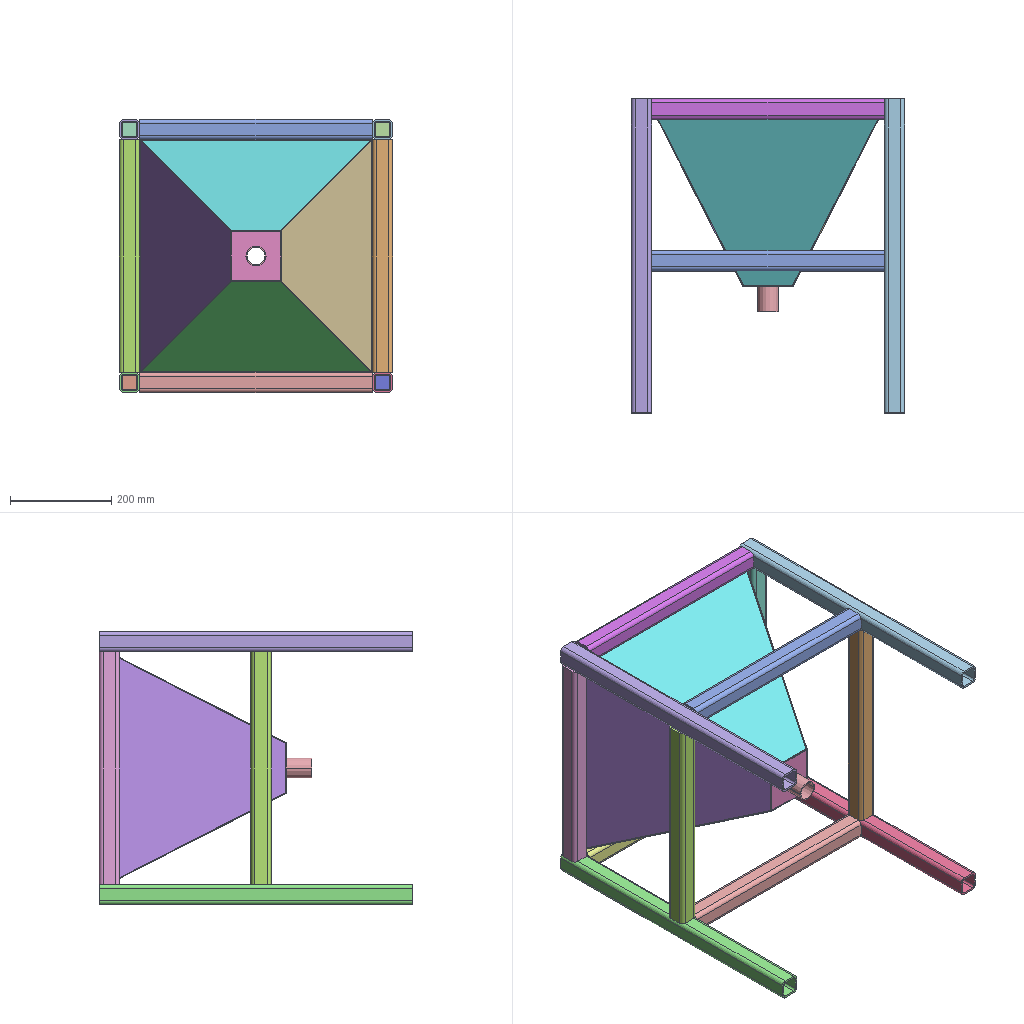Assembly | SolidWorks | 7 different items | 7 placed | box 540 x 620 x 540 mm
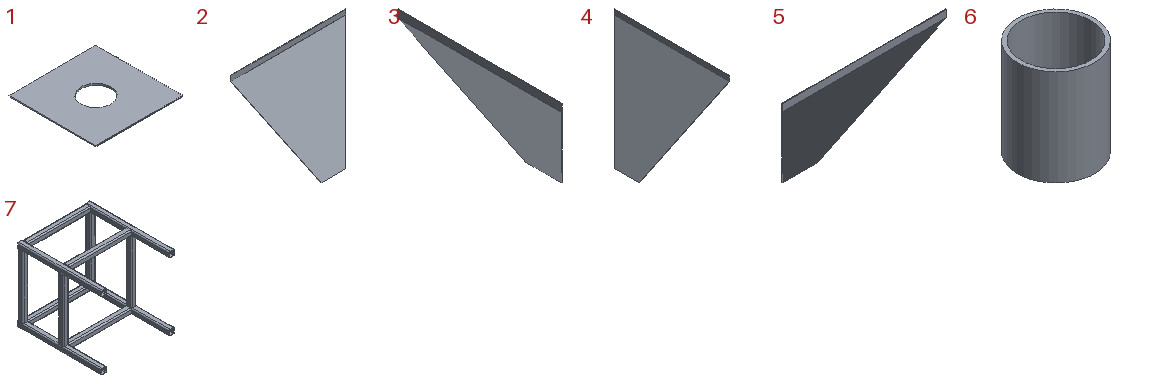Parts list (item | quantity | size | volume | features):
1 | x1 | 102.046 x 102.046 x 2 mm | 18488 mm3 | features ICE 3, DeleteBody 2, Split 2, Blend 1, Shell 1
2 | x1 | 454 x 180.224 x 368.911 mm | 234028 mm3 | features ICE 3, Blend 1, FlatPattern 1, SheetMetal 1, Shell 1, SolidToSheetMetal 1
3 | x1 | 180.781 x 458 x 370 mm | 237222 mm3 | features ICE 3, Blend 1, FlatPattern 1, SheetMetal 1, Shell 1, SolidToSheetMetal 1
4 | x1 | 180.781 x 458 x 370 mm | 237222 mm3 | features ICE 3, Blend 1, FlatPattern 1, SheetMetal 1, Shell 1, SolidToSheetMetal 1
5 | x1 | 454 x 180.224 x 368.911 mm | 234028 mm3 | features ICE 3, Blend 1, FlatPattern 1, SheetMetal 1, Shell 1, SolidToSheetMetal 1
6 | x1 | 40 x 40 x 50 mm | 11938 mm3 | features ICE 3, DeleteBody 2, Split 2, Blend 1, Shell 1
7 | x1 | 540 x 620 x 540 mm | 3300618 mm3 | features WeldCornerFeat 2, 3DProfileFeature 1, EndCap 1, WeldMemberFeat 1, WeldmentFeature 1
Mates (type | each side: item.copy, entity, surface, feature):
Coordinate | 7.1 select_type:25 | assembly select_type:11
Coordinate | 2.1 select_type:25 | 3.1 select_type:25
Coordinate | 4.1 select_type:25 | 5.1 select_type:25
Coordinate | 3.1 select_type:25 | 4.1 select_type:25
Coordinate | 1.1 select_type:25 | 4.1 select_type:25
Symmetric | 3.1 face plane Convert entities1 | 4.1 face plane Convert entities1 | assembly plane
Symmetric | 2.1 face plane Convert entities1 | 5.1 face plane Convert entities4 | assembly plane
Coincident | 7.1 face plane Square tube 40 X 40 X 4(1) | 5.1 edge
Concentric | 1.1 edge | 6.1 edge
Coincident | 1.1 face plane Loft1 | 6.1 edge